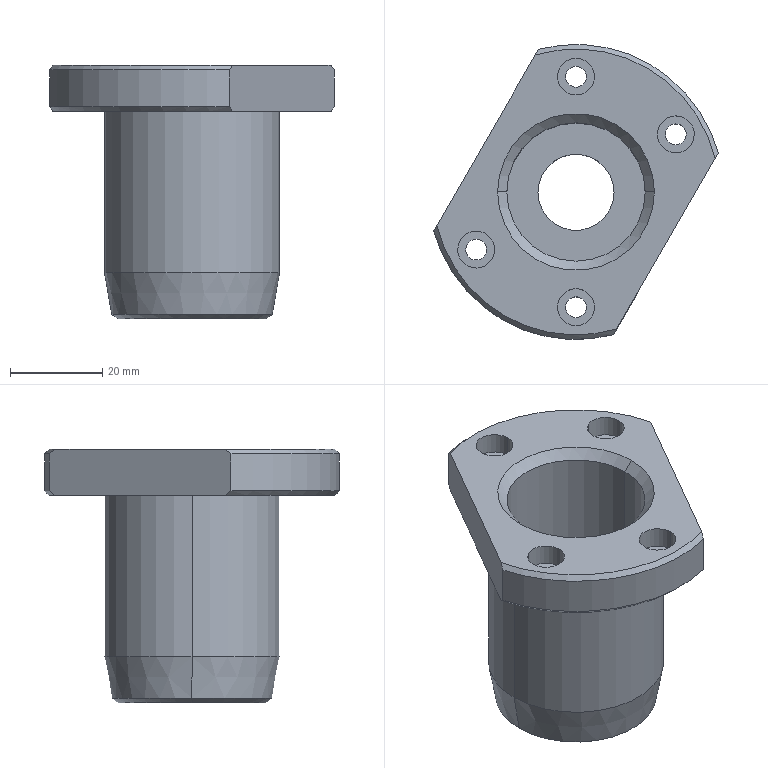Part | SolidWorks | features Chamfer 4, ICE 3, 3DProfileFeature 2, HoleWzd 2, CirPattern 1, Extrusion 1 | 1 solid | 44 faces | box 61.725 x 64 x 55 mm | volume 43113 mm3 | cylinder 24 | cone 10 | plane 10 | commonest cylinder face diameters 4.5 x8 8 x8 16.5 x2 30 x2 38 x2 64 x2
STEP:
#1=CARTESIAN_POINT('',(-15.,0.,53.));
#2=VERTEX_POINT('',#1);
#3=CARTESIAN_POINT('',(15.,0.,53.));
#4=VERTEX_POINT('',#3);
#5=CARTESIAN_POINT('',(0.,0.,53.));
#6=DIRECTION('',(0.,0.,1.));
#7=DIRECTION('',(1.,0.,0.));
#8=AXIS2_PLACEMENT_3D('',#5,#6,#7);
#9=CIRCLE('',#8,15.);
#10=EDGE_CURVE('',#2,#4,#9,.T.);
#11=ORIENTED_EDGE('',*,*,#10,.F.);
#12=CARTESIAN_POINT('',(-17.,0.,55.));
#13=VERTEX_POINT('',#12);
#14=CARTESIAN_POINT('',(-15.,0.,53.));
#15=DIRECTION('',(-0.7071,0.,0.7071));
#16=VECTOR('',#15,1000.);
#17=LINE('',#14,#16);
#18=EDGE_CURVE('',#2,#13,#17,.T.);
#19=ORIENTED_EDGE('',*,*,#18,.T.);
#20=CARTESIAN_POINT('',(17.,0.,55.));
#21=VERTEX_POINT('',#20);
#22=CARTESIAN_POINT('',(0.,0.,55.));
#23=DIRECTION('',(0.,0.,-1.));
#24=DIRECTION('',(1.,0.,0.));
#25=AXIS2_PLACEMENT_3D('',#22,#23,#24);
#26=CIRCLE('',#25,17.);
#27=EDGE_CURVE('',#21,#13,#26,.T.);
#28=ORIENTED_EDGE('',*,*,#27,.F.);
#29=CARTESIAN_POINT('',(15.,0.,53.));
#30=DIRECTION('',(0.7071,0.,0.7071));
#31=VECTOR('',#30,1000.);
#32=LINE('',#29,#31);
#33=EDGE_CURVE('',#4,#21,#32,.T.);
#34=ORIENTED_EDGE('',*,*,#33,.F.);
#35=EDGE_LOOP('',(#11,#19,#28,#34));
#36=FACE_OUTER_BOUND('',#35,.T.);
#37=CARTESIAN_POINT('',(0.,0.,53.));
#38=DIRECTION('',(0.,0.,1.));
#39=DIRECTION('',(1.,0.,0.));
#40=AXIS2_PLACEMENT_3D('',#37,#38,#39);
#41=CONICAL_SURFACE('',#40,15.,0.7854);
#42=ADVANCED_FACE('',(#36),#41,.F.);
#43=CARTESIAN_POINT('',(-16.004,0.,0.));
#44=VERTEX_POINT('',#43);
#45=CARTESIAN_POINT('',(16.004,0.,0.));
#46=VERTEX_POINT('',#45);
#47=CARTESIAN_POINT('',(0.,0.,0.));
#48=DIRECTION('',(0.,0.,-1.));
#49=DIRECTION('',(1.,0.,0.));
#50=AXIS2_PLACEMENT_3D('',#47,#48,#49);
#51=CIRCLE('',#50,16.004);
#52=EDGE_CURVE('',#44,#46,#51,.T.);
#53=ORIENTED_EDGE('',*,*,#52,.F.);
#54=CARTESIAN_POINT('',(-17.41,0.,0.9848));
#55=VERTEX_POINT('',#54);
#56=CARTESIAN_POINT('',(-16.004,0.,0.));
#57=DIRECTION('',(-0.8192,0.,0.5736));
#58=VECTOR('',#57,1000.);
#59=LINE('',#56,#58);
#60=EDGE_CURVE('',#44,#55,#59,.T.);
#61=ORIENTED_EDGE('',*,*,#60,.T.);
#62=CARTESIAN_POINT('',(17.41,0.,0.9848));
#63=VERTEX_POINT('',#62);
#64=CARTESIAN_POINT('',(0.,0.,0.9848));
#65=DIRECTION('',(0.,0.,1.));
#66=DIRECTION('',(1.,0.,0.));
#67=AXIS2_PLACEMENT_3D('',#64,#65,#66);
#68=CIRCLE('',#67,17.41);
#69=EDGE_CURVE('',#63,#55,#68,.T.);
#70=ORIENTED_EDGE('',*,*,#69,.F.);
#71=CARTESIAN_POINT('',(16.004,0.,0.));
#72=DIRECTION('',(0.8192,0.,0.5736));
#73=VECTOR('',#72,1000.);
#74=LINE('',#71,#73);
#75=EDGE_CURVE('',#46,#63,#74,.T.);
#76=ORIENTED_EDGE('',*,*,#75,.F.);
#77=EDGE_LOOP('',(#53,#61,#70,#76));
#78=FACE_OUTER_BOUND('',#77,.T.);
#79=CARTESIAN_POINT('',(0.,0.,0.));
#80=DIRECTION('',(0.,0.,1.));
#81=DIRECTION('',(1.,0.,0.));
#82=AXIS2_PLACEMENT_3D('',#79,#80,#81);
#83=CONICAL_SURFACE('',#82,16.004,0.9599);
#84=ADVANCED_FACE('',(#78),#83,.T.);
#85=ORIENTED_EDGE('',*,*,#69,.T.);
#86=CARTESIAN_POINT('',(-19.,0.,10.));
#87=VERTEX_POINT('',#86);
#88=CARTESIAN_POINT('',(-19.,0.,10.));
#89=DIRECTION('',(-0.1736,0.,0.9848));
#90=VECTOR('',#89,1000.);
#91=LINE('',#88,#90);
#92=EDGE_CURVE('',#55,#87,#91,.T.);
#93=ORIENTED_EDGE('',*,*,#92,.T.);
#94=CARTESIAN_POINT('',(19.,0.,10.));
#95=VERTEX_POINT('',#94);
#96=CARTESIAN_POINT('',(0.,0.,10.));
#97=DIRECTION('',(0.,0.,1.));
#98=DIRECTION('',(1.,0.,0.));
#99=AXIS2_PLACEMENT_3D('',#96,#97,#98);
#100=CIRCLE('',#99,19.);
#101=EDGE_CURVE('',#95,#87,#100,.T.);
#102=ORIENTED_EDGE('',*,*,#101,.F.);
#103=CARTESIAN_POINT('',(19.,0.,10.));
#104=DIRECTION('',(0.1736,0.,0.9848));
#105=VECTOR('',#104,1000.);
#106=LINE('',#103,#105);
#107=EDGE_CURVE('',#63,#95,#106,.T.);
#108=ORIENTED_EDGE('',*,*,#107,.F.);
#109=EDGE_LOOP('',(#85,#93,#102,#108));
#110=FACE_OUTER_BOUND('',#109,.T.);
#111=CARTESIAN_POINT('',(0.,0.,10.));
#112=DIRECTION('',(0.,0.,1.));
#113=DIRECTION('',(1.,0.,0.));
#114=AXIS2_PLACEMENT_3D('',#111,#112,#113);
#115=CONICAL_SURFACE('',#114,19.,0.1745);
#116=ADVANCED_FACE('',(#110),#115,.T.);
#117=CARTESIAN_POINT('',(19.651,15.964,50.4));
#118=VERTEX_POINT('',#117);
#119=CARTESIAN_POINT('',(23.651,9.036,50.4));
#120=VERTEX_POINT('',#119);
#121=CARTESIAN_POINT('',(21.651,12.5,50.4));
#122=DIRECTION('',(0.,0.,1.));
#123=DIRECTION('',(0.5,-0.866,0.));
#124=AXIS2_PLACEMENT_3D('',#121,#122,#123);
#125=CIRCLE('',#124,4.);
#126=EDGE_CURVE('',#118,#120,#125,.T.);
#127=ORIENTED_EDGE('',*,*,#126,.F.);
#128=CARTESIAN_POINT('',(19.651,15.964,55.));
#129=VERTEX_POINT('',#128);
#130=CARTESIAN_POINT('',(19.651,15.964,55.));
#131=DIRECTION('',(0.,0.,1.));
#132=VECTOR('',#131,1000.);
#133=LINE('',#130,#132);
#134=EDGE_CURVE('',#118,#129,#133,.T.);
#135=ORIENTED_EDGE('',*,*,#134,.T.);
#136=CARTESIAN_POINT('',(23.651,9.036,55.));
#137=VERTEX_POINT('',#136);
#138=CARTESIAN_POINT('',(21.651,12.5,55.));
#139=DIRECTION('',(0.,0.,1.));
#140=DIRECTION('',(0.5,-0.866,0.));
#141=AXIS2_PLACEMENT_3D('',#138,#139,#140);
#142=CIRCLE('',#141,4.);
#143=EDGE_CURVE('',#129,#137,#142,.T.);
#144=ORIENTED_EDGE('',*,*,#143,.T.);
#145=CARTESIAN_POINT('',(23.651,9.036,55.));
#146=DIRECTION('',(0.,0.,1.));
#147=VECTOR('',#146,1000.);
#148=LINE('',#145,#147);
#149=EDGE_CURVE('',#120,#137,#148,.T.);
#150=ORIENTED_EDGE('',*,*,#149,.F.);
#151=EDGE_LOOP('',(#127,#135,#144,#150));
#152=FACE_OUTER_BOUND('',#151,.T.);
#153=CARTESIAN_POINT('',(21.651,12.5,55.));
#154=DIRECTION('',(0.,0.,1.));
#155=DIRECTION('',(0.5,-0.866,0.));
#156=AXIS2_PLACEMENT_3D('',#153,#154,#155);
#157=CYLINDRICAL_SURFACE('',#156,4.);
#158=ADVANCED_FACE('',(#152),#157,.F.);
#159=CARTESIAN_POINT('',(20.526,14.449,45.));
#160=VERTEX_POINT('',#159);
#161=CARTESIAN_POINT('',(22.776,10.551,45.));
#162=VERTEX_POINT('',#161);
#163=CARTESIAN_POINT('',(21.651,12.5,45.));
#164=DIRECTION('',(0.,0.,1.));
#165=DIRECTION('',(0.5,-0.866,0.));
#166=AXIS2_PLACEMENT_3D('',#163,#164,#165);
#167=CIRCLE('',#166,2.25);
#168=EDGE_CURVE('',#160,#162,#167,.T.);
#169=ORIENTED_EDGE('',*,*,#168,.F.);
#170=CARTESIAN_POINT('',(20.526,14.449,50.4));
#171=VERTEX_POINT('',#170);
#172=CARTESIAN_POINT('',(20.526,14.449,55.));
#173=DIRECTION('',(0.,0.,1.));
#174=VECTOR('',#173,1000.);
#175=LINE('',#172,#174);
#176=EDGE_CURVE('',#160,#171,#175,.T.);
#177=ORIENTED_EDGE('',*,*,#176,.T.);
#178=CARTESIAN_POINT('',(22.776,10.551,50.4));
#179=VERTEX_POINT('',#178);
#180=CARTESIAN_POINT('',(21.651,12.5,50.4));
#181=DIRECTION('',(0.,0.,1.));
#182=DIRECTION('',(0.5,-0.866,0.));
#183=AXIS2_PLACEMENT_3D('',#180,#181,#182);
#184=CIRCLE('',#183,2.25);
#185=EDGE_CURVE('',#171,#179,#184,.T.);
#186=ORIENTED_EDGE('',*,*,#185,.T.);
#187=CARTESIAN_POINT('',(22.776,10.551,55.));
#188=DIRECTION('',(0.,0.,1.));
#189=VECTOR('',#188,1000.);
#190=LINE('',#187,#189);
#191=EDGE_CURVE('',#162,#179,#190,.T.);
#192=ORIENTED_EDGE('',*,*,#191,.F.);
#193=EDGE_LOOP('',(#169,#177,#186,#192));
#194=FACE_OUTER_BOUND('',#193,.T.);
#195=CARTESIAN_POINT('',(21.651,12.5,55.));
#196=DIRECTION('',(0.,0.,1.));
#197=DIRECTION('',(0.5,-0.866,0.));
#198=AXIS2_PLACEMENT_3D('',#195,#196,#197);
#199=CYLINDRICAL_SURFACE('',#198,2.25);
#200=ADVANCED_FACE('',(#194),#199,.F.);
#201=CARTESIAN_POINT('',(4.,-25.,50.4));
#202=VERTEX_POINT('',#201);
#203=CARTESIAN_POINT('',(-4.,-25.,50.4));
#204=VERTEX_POINT('',#203);
#205=CARTESIAN_POINT('',(0.,-25.,50.4));
#206=DIRECTION('',(0.,0.,1.));
#207=DIRECTION('',(-1.,0.,0.));
#208=AXIS2_PLACEMENT_3D('',#205,#206,#207);
#209=CIRCLE('',#208,4.);
#210=EDGE_CURVE('',#202,#204,#209,.T.);
#211=ORIENTED_EDGE('',*,*,#210,.F.);
#212=CARTESIAN_POINT('',(4.,-25.,55.));
#213=VERTEX_POINT('',#212);
#214=CARTESIAN_POINT('',(4.,-25.,55.));
#215=DIRECTION('',(0.,0.,1.));
#216=VECTOR('',#215,1000.);
#217=LINE('',#214,#216);
#218=EDGE_CURVE('',#202,#213,#217,.T.);
#219=ORIENTED_EDGE('',*,*,#218,.T.);
#220=CARTESIAN_POINT('',(-4.,-25.,55.));
#221=VERTEX_POINT('',#220);
#222=CARTESIAN_POINT('',(0.,-25.,55.));
#223=DIRECTION('',(0.,0.,1.));
#224=DIRECTION('',(-1.,0.,0.));
#225=AXIS2_PLACEMENT_3D('',#222,#223,#224);
#226=CIRCLE('',#225,4.);
#227=EDGE_CURVE('',#213,#221,#226,.T.);
#228=ORIENTED_EDGE('',*,*,#227,.T.);
#229=CARTESIAN_POINT('',(-4.,-25.,55.));
#230=DIRECTION('',(0.,0.,1.));
#231=VECTOR('',#230,1000.);
#232=LINE('',#229,#231);
#233=EDGE_CURVE('',#204,#221,#232,.T.);
#234=ORIENTED_EDGE('',*,*,#233,.F.);
#235=EDGE_LOOP('',(#211,#219,#228,#234));
#236=FACE_OUTER_BOUND('',#235,.T.);
#237=CARTESIAN_POINT('',(0.,-25.,55.));
#238=DIRECTION('',(0.,0.,1.));
#239=DIRECTION('',(-1.,0.,0.));
#240=AXIS2_PLACEMENT_3D('',#237,#238,#239);
#241=CYLINDRICAL_SURFACE('',#240,4.);
#242=ADVANCED_FACE('',(#236),#241,.F.);
#243=CARTESIAN_POINT('',(2.25,-25.,45.));
#244=VERTEX_POINT('',#243);
#245=CARTESIAN_POINT('',(-2.25,-25.,45.));
#246=VERTEX_POINT('',#245);
#247=CARTESIAN_POINT('',(0.,-25.,45.));
#248=DIRECTION('',(0.,0.,1.));
#249=DIRECTION('',(-1.,0.,0.));
#250=AXIS2_PLACEMENT_3D('',#247,#248,#249);
#251=CIRCLE('',#250,2.25);
#252=EDGE_CURVE('',#244,#246,#251,.T.);
#253=ORIENTED_EDGE('',*,*,#252,.F.);
#254=CARTESIAN_POINT('',(2.25,-25.,50.4));
#255=VERTEX_POINT('',#254);
#256=CARTESIAN_POINT('',(2.25,-25.,55.));
#257=DIRECTION('',(0.,0.,1.));
#258=VECTOR('',#257,1000.);
#259=LINE('',#256,#258);
#260=EDGE_CURVE('',#244,#255,#259,.T.);
#261=ORIENTED_EDGE('',*,*,#260,.T.);
#262=CARTESIAN_POINT('',(-2.25,-25.,50.4));
#263=VERTEX_POINT('',#262);
#264=CARTESIAN_POINT('',(0.,-25.,50.4));
#265=DIRECTION('',(0.,0.,1.));
#266=DIRECTION('',(-1.,0.,0.));
#267=AXIS2_PLACEMENT_3D('',#264,#265,#266);
#268=CIRCLE('',#267,2.25);
#269=EDGE_CURVE('',#255,#263,#268,.T.);
#270=ORIENTED_EDGE('',*,*,#269,.T.);
#271=CARTESIAN_POINT('',(-2.25,-25.,55.));
#272=DIRECTION('',(0.,0.,1.));
#273=VECTOR('',#272,1000.);
#274=LINE('',#271,#273);
#275=EDGE_CURVE('',#246,#263,#274,.T.);
#276=ORIENTED_EDGE('',*,*,#275,.F.);
#277=EDGE_LOOP('',(#253,#261,#270,#276));
#278=FACE_OUTER_BOUND('',#277,.T.);
#279=CARTESIAN_POINT('',(0.,-25.,55.));
#280=DIRECTION('',(0.,0.,1.));
#281=DIRECTION('',(-1.,0.,0.));
#282=AXIS2_PLACEMENT_3D('',#279,#280,#281);
#283=CYLINDRICAL_SURFACE('',#282,2.25);
#284=ADVANCED_FACE('',(#278),#283,.F.);
#285=CARTESIAN_POINT('',(-19.651,-15.964,50.4));
#286=VERTEX_POINT('',#285);
#287=CARTESIAN_POINT('',(-23.651,-9.036,50.4));
#288=VERTEX_POINT('',#287);
#289=CARTESIAN_POINT('',(-21.651,-12.5,50.4));
#290=DIRECTION('',(0.,0.,1.));
#291=DIRECTION('',(-0.5,0.866,0.));
#292=AXIS2_PLACEMENT_3D('',#289,#290,#291);
#293=CIRCLE('',#292,4.);
#294=EDGE_CURVE('',#286,#288,#293,.T.);
#295=ORIENTED_EDGE('',*,*,#294,.F.);
#296=CARTESIAN_POINT('',(-19.651,-15.964,55.));
#297=VERTEX_POINT('',#296);
#298=CARTESIAN_POINT('',(-19.651,-15.964,55.));
#299=DIRECTION('',(0.,0.,1.));
#300=VECTOR('',#299,1000.);
#301=LINE('',#298,#300);
#302=EDGE_CURVE('',#286,#297,#301,.T.);
#303=ORIENTED_EDGE('',*,*,#302,.T.);
#304=CARTESIAN_POINT('',(-23.651,-9.036,55.));
#305=VERTEX_POINT('',#304);
#306=CARTESIAN_POINT('',(-21.651,-12.5,55.));
#307=DIRECTION('',(0.,0.,1.));
#308=DIRECTION('',(-0.5,0.866,0.));
#309=AXIS2_PLACEMENT_3D('',#306,#307,#308);
#310=CIRCLE('',#309,4.);
#311=EDGE_CURVE('',#297,#305,#310,.T.);
#312=ORIENTED_EDGE('',*,*,#311,.T.);
#313=CARTESIAN_POINT('',(-23.651,-9.036,55.));
#314=DIRECTION('',(0.,0.,1.));
#315=VECTOR('',#314,1000.);
#316=LINE('',#313,#315);
#317=EDGE_CURVE('',#288,#305,#316,.T.);
#318=ORIENTED_EDGE('',*,*,#317,.F.);
#319=EDGE_LOOP('',(#295,#303,#312,#318));
#320=FACE_OUTER_BOUND('',#319,.T.);
#321=CARTESIAN_POINT('',(-21.651,-12.5,55.));
#322=DIRECTION('',(0.,0.,1.));
#323=DIRECTION('',(-0.5,0.866,0.));
#324=AXIS2_PLACEMENT_3D('',#321,#322,#323);
#325=CYLINDRICAL_SURFACE('',#324,4.);
#326=ADVANCED_FACE('',(#320),#325,.F.);
#327=CARTESIAN_POINT('',(-20.526,-14.449,45.));
#328=VERTEX_POINT('',#327);
#329=CARTESIAN_POINT('',(-22.776,-10.551,45.));
#330=VERTEX_POINT('',#329);
#331=CARTESIAN_POINT('',(-21.651,-12.5,45.));
#332=DIRECTION('',(0.,0.,1.));
#333=DIRECTION('',(-0.5,0.866,0.));
#334=AXIS2_PLACEMENT_3D('',#331,#332,#333);
#335=CIRCLE('',#334,2.25);
#336=EDGE_CURVE('',#328,#330,#335,.T.);
#337=ORIENTED_EDGE('',*,*,#336,.F.);
#338=CARTESIAN_POINT('',(-20.526,-14.449,50.4));
#339=VERTEX_POINT('',#338);
#340=CARTESIAN_POINT('',(-20.526,-14.449,55.));
#341=DIRECTION('',(0.,0.,1.));
#342=VECTOR('',#341,1000.);
#343=LINE('',#340,#342);
#344=EDGE_CURVE('',#328,#339,#343,.T.);
#345=ORIENTED_EDGE('',*,*,#344,.T.);
#346=CARTESIAN_POINT('',(-22.776,-10.551,50.4));
#347=VERTEX_POINT('',#346);
#348=CARTESIAN_POINT('',(-21.651,-12.5,50.4));
#349=DIRECTION('',(0.,0.,1.));
#350=DIRECTION('',(-0.5,0.866,0.));
#351=AXIS2_PLACEMENT_3D('',#348,#349,#350);
#352=CIRCLE('',#351,2.25);
#353=EDGE_CURVE('',#339,#347,#352,.T.);
#354=ORIENTED_EDGE('',*,*,#353,.T.);
#355=CARTESIAN_POINT('',(-22.776,-10.551,55.));
#356=DIRECTION('',(0.,0.,1.));
#357=VECTOR('',#356,1000.);
#358=LINE('',#355,#357);
#359=EDGE_CURVE('',#330,#347,#358,.T.);
#360=ORIENTED_EDGE('',*,*,#359,.F.);
#361=EDGE_LOOP('',(#337,#345,#354,#360));
#362=FACE_OUTER_BOUND('',#361,.T.);
#363=CARTESIAN_POINT('',(-21.651,-12.5,55.));
#364=DIRECTION('',(0.,0.,1.));
#365=DIRECTION('',(-0.5,0.866,0.));
#366=AXIS2_PLACEMENT_3D('',#363,#364,#365);
#367=CYLINDRICAL_SURFACE('',#366,2.25);
#368=ADVANCED_FACE('',(#362),#367,.F.);
#369=CARTESIAN_POINT('',(-4.,25.,50.4));
#370=VERTEX_POINT('',#369);
#371=CARTESIAN_POINT('',(4.,25.,50.4));
#372=VERTEX_POINT('',#371);
#373=CARTESIAN_POINT('',(0.,25.,50.4));
#374=DIRECTION('',(0.,0.,1.));
#375=DIRECTION('',(1.,0.,0.));
#376=AXIS2_PLACEMENT_3D('',#373,#374,#375);
#377=CIRCLE('',#376,4.);
#378=EDGE_CURVE('',#370,#372,#377,.T.);
#379=ORIENTED_EDGE('',*,*,#378,.F.);
#380=CARTESIAN_POINT('',(-4.,25.,55.));
#381=VERTEX_POINT('',#380);
#382=CARTESIAN_POINT('',(-4.,25.,55.));
#383=DIRECTION('',(0.,0.,1.));
#384=VECTOR('',#383,1000.);
#385=LINE('',#382,#384);
#386=EDGE_CURVE('',#370,#381,#385,.T.);
#387=ORIENTED_EDGE('',*,*,#386,.T.);
#388=CARTESIAN_POINT('',(4.,25.,55.));
#389=VERTEX_POINT('',#388);
#390=CARTESIAN_POINT('',(0.,25.,55.));
#391=DIRECTION('',(0.,0.,1.));
#392=DIRECTION('',(1.,0.,0.));
#393=AXIS2_PLACEMENT_3D('',#390,#391,#392);
#394=CIRCLE('',#393,4.);
#395=EDGE_CURVE('',#381,#389,#394,.T.);
#396=ORIENTED_EDGE('',*,*,#395,.T.);
#397=CARTESIAN_POINT('',(4.,25.,55.));
#398=DIRECTION('',(0.,0.,1.));
#399=VECTOR('',#398,1000.);
#400=LINE('',#397,#399);
#401=EDGE_CURVE('',#372,#389,#400,.T.);
#402=ORIENTED_EDGE('',*,*,#401,.F.);
#403=EDGE_LOOP('',(#379,#387,#396,#402));
#404=FACE_OUTER_BOUND('',#403,.T.);
#405=CARTESIAN_POINT('',(0.,25.,55.));
#406=DIRECTION('',(0.,0.,1.));
#407=DIRECTION('',(1.,0.,0.));
#408=AXIS2_PLACEMENT_3D('',#405,#406,#407);
#409=CYLINDRICAL_SURFACE('',#408,4.);
#410=ADVANCED_FACE('',(#404),#409,.F.);
#411=CARTESIAN_POINT('',(-2.25,25.,45.));
#412=VERTEX_POINT('',#411);
#413=CARTESIAN_POINT('',(2.25,25.,45.));
#414=VERTEX_POINT('',#413);
#415=CARTESIAN_POINT('',(0.,25.,45.));
#416=DIRECTION('',(0.,0.,1.));
#417=DIRECTION('',(1.,0.,0.));
#418=AXIS2_PLACEMENT_3D('',#415,#416,#417);
#419=CIRCLE('',#418,2.25);
#420=EDGE_CURVE('',#412,#414,#419,.T.);
#421=ORIENTED_EDGE('',*,*,#420,.F.);
#422=CARTESIAN_POINT('',(-2.25,25.,50.4));
#423=VERTEX_POINT('',#422);
#424=CARTESIAN_POINT('',(-2.25,25.,55.));
#425=DIRECTION('',(0.,0.,1.));
#426=VECTOR('',#425,1000.);
#427=LINE('',#424,#426);
#428=EDGE_CURVE('',#412,#423,#427,.T.);
#429=ORIENTED_EDGE('',*,*,#428,.T.);
#430=CARTESIAN_POINT('',(2.25,25.,50.4));
#431=VERTEX_POINT('',#430);
#432=CARTESIAN_POINT('',(0.,25.,50.4));
#433=DIRECTION('',(0.,0.,1.));
#434=DIRECTION('',(1.,0.,0.));
#435=AXIS2_PLACEMENT_3D('',#432,#433,#434);
#436=CIRCLE('',#435,2.25);
#437=EDGE_CURVE('',#423,#431,#436,.T.);
#438=ORIENTED_EDGE('',*,*,#437,.T.);
#439=CARTESIAN_POINT('',(2.25,25.,55.));
#440=DIRECTION('',(0.,0.,1.));
#441=VECTOR('',#440,1000.);
#442=LINE('',#439,#441);
#443=EDGE_CURVE('',#414,#431,#442,.T.);
#444=ORIENTED_EDGE('',*,*,#443,.F.);
#445=EDGE_LOOP('',(#421,#429,#438,#444));
#446=FACE_OUTER_BOUND('',#445,.T.);
#447=CARTESIAN_POINT('',(0.,25.,55.));
#448=DIRECTION('',(0.,0.,1.));
#449=DIRECTION('',(1.,0.,0.));
#450=AXIS2_PLACEMENT_3D('',#447,#448,#449);
#451=CYLINDRICAL_SURFACE('',#450,2.25);
#452=ADVANCED_FACE('',(#446),#451,.F.);
#453=CARTESIAN_POINT('',(-8.25,0.,15.));
#454=VERTEX_POINT('',#453);
#455=CARTESIAN_POINT('',(8.25,0.,15.));
#456=VERTEX_POINT('',#455);
#457=CARTESIAN_POINT('',(0.,0.,15.));
#458=DIRECTION('',(0.,0.,1.));
#459=DIRECTION('',(1.,0.,0.));
#460=AXIS2_PLACEMENT_3D('',#457,#458,#459);
#461=CIRCLE('',#460,8.25);
#462=EDGE_CURVE('',#454,#456,#461,.T.);
#463=ORIENTED_EDGE('',*,*,#462,.T.);
#464=CARTESIAN_POINT('',(8.25,0.,0.));
#465=VERTEX_POINT('',#464);
#466=CARTESIAN_POINT('',(8.25,0.,0.));
#467=DIRECTION('',(0.,0.,-1.));
#468=VECTOR('',#467,1000.);
#469=LINE('',#466,#468);
#470=EDGE_CURVE('',#456,#465,#469,.T.);
#471=ORIENTED_EDGE('',*,*,#470,.T.);
#472=CARTESIAN_POINT('',(-8.25,0.,0.));
#473=VERTEX_POINT('',#472);
#474=CARTESIAN_POINT('',(0.,0.,0.));
#475=DIRECTION('',(0.,0.,-1.));
#476=DIRECTION('',(-1.,0.,0.));
#477=AXIS2_PLACEMENT_3D('',#474,#475,#476);
#478=CIRCLE('',#477,8.25);
#479=EDGE_CURVE('',#465,#473,#478,.T.);
#480=ORIENTED_EDGE('',*,*,#479,.T.);
#481=CARTESIAN_POINT('',(-8.25,0.,0.));
#482=DIRECTION('',(0.,0.,-1.));
#483=VECTOR('',#482,1000.);
#484=LINE('',#481,#483);
#485=EDGE_CURVE('',#454,#473,#484,.T.);
#486=ORIENTED_EDGE('',*,*,#485,.F.);
#487=EDGE_LOOP('',(#463,#471,#480,#486));
#488=FACE_OUTER_BOUND('',#487,.T.);
#489=CARTESIAN_POINT('',(0.,0.,0.));
#490=DIRECTION('',(0.,0.,-1.));
#491=DIRECTION('',(-1.,0.,0.));
#492=AXIS2_PLACEMENT_3D('',#489,#490,#491);
#493=CYLINDRICAL_SURFACE('',#492,8.25);
#494=ADVANCED_FACE('',(#488),#493,.F.);
#495=CARTESIAN_POINT('',(15.,0.,15.));
#496=VERTEX_POINT('',#495);
#497=CARTESIAN_POINT('',(-15.,0.,15.));
#498=VERTEX_POINT('',#497);
#499=CARTESIAN_POINT('',(0.,0.,15.));
#500=DIRECTION('',(0.,0.,-1.));
#501=DIRECTION('',(1.,0.,0.));
#502=AXIS2_PLACEMENT_3D('',#499,#500,#501);
#503=CIRCLE('',#502,15.);
#504=EDGE_CURVE('',#496,#498,#503,.T.);
#505=ORIENTED_EDGE('',*,*,#504,.T.);
#506=CARTESIAN_POINT('',(-15.,0.,-42.426));
#507=DIRECTION('',(0.,0.,1.));
#508=VECTOR('',#507,1000.);
#509=LINE('',#506,#508);
#510=EDGE_CURVE('',#498,#2,#509,.T.);
#511=ORIENTED_EDGE('',*,*,#510,.T.);
#512=ORIENTED_EDGE('',*,*,#10,.T.);
#513=CARTESIAN_POINT('',(15.,0.,-42.426));
#514=DIRECTION('',(0.,0.,1.));
#515=VECTOR('',#514,1000.);
#516=LINE('',#513,#515);
#517=EDGE_CURVE('',#496,#4,#516,.T.);
#518=ORIENTED_EDGE('',*,*,#517,.F.);
#519=EDGE_LOOP('',(#505,#511,#512,#518));
#520=FACE_OUTER_BOUND('',#519,.T.);
#521=CARTESIAN_POINT('',(0.,0.,-42.426));
#522=DIRECTION('',(0.,0.,1.));
#523=DIRECTION('',(1.,0.,0.));
#524=AXIS2_PLACEMENT_3D('',#521,#522,#523);
#525=CYLINDRICAL_SURFACE('',#524,15.);
#526=ADVANCED_FACE('',(#520),#525,.F.);
#527=CARTESIAN_POINT('',(19.,0.,45.));
#528=VERTEX_POINT('',#527);
#529=CARTESIAN_POINT('',(-19.,0.,45.));
#530=VERTEX_POINT('',#529);
#531=CARTESIAN_POINT('',(0.,0.,45.));
#532=DIRECTION('',(0.,0.,1.));
#533=DIRECTION('',(1.,0.,0.));
#534=AXIS2_PLACEMENT_3D('',#531,#532,#533);
#535=CIRCLE('',#534,19.);
#536=EDGE_CURVE('',#528,#530,#535,.T.);
#537=ORIENTED_EDGE('',*,*,#536,.F.);
#538=CARTESIAN_POINT('',(19.,0.,45.));
#539=DIRECTION('',(0.,0.,-1.));
#540=VECTOR('',#539,1000.);
#541=LINE('',#538,#540);
#542=EDGE_CURVE('',#528,#95,#541,.T.);
#543=ORIENTED_EDGE('',*,*,#542,.T.);
#544=ORIENTED_EDGE('',*,*,#101,.T.);
#545=CARTESIAN_POINT('',(-19.,0.,45.));
#546=DIRECTION('',(0.,0.,-1.));
#547=VECTOR('',#546,1000.);
#548=LINE('',#545,#547);
#549=EDGE_CURVE('',#530,#87,#548,.T.);
#550=ORIENTED_EDGE('',*,*,#549,.F.);
#551=EDGE_LOOP('',(#537,#543,#544,#550));
#552=FACE_OUTER_BOUND('',#551,.T.);
#553=CARTESIAN_POINT('',(0.,0.,45.));
#554=DIRECTION('',(0.,0.,-1.));
#555=DIRECTION('',(-1.,0.,0.));
#556=AXIS2_PLACEMENT_3D('',#553,#554,#555);
#557=CYLINDRICAL_SURFACE('',#556,19.);
#558=ADVANCED_FACE('',(#552),#557,.T.);
#559=CARTESIAN_POINT('',(30.863,8.456,46.));
#560=VERTEX_POINT('',#559);
#561=CARTESIAN_POINT('',(30.863,8.456,54.));
#562=VERTEX_POINT('',#561);
#563=CARTESIAN_POINT('',(30.863,8.456,-0.001));
#564=DIRECTION('',(0.,0.,1.));
#565=VECTOR('',#564,1000.);
#566=LINE('',#563,#565);
#567=EDGE_CURVE('',#560,#562,#566,.T.);
#568=ORIENTED_EDGE('',*,*,#567,.F.);
#569=CARTESIAN_POINT('',(-8.109,30.956,46.));
#570=VERTEX_POINT('',#569);
#571=CARTESIAN_POINT('',(0.,0.,46.));
#572=DIRECTION('',(0.,0.,1.));
#573=DIRECTION('',(1.,0.,0.));
#574=AXIS2_PLACEMENT_3D('',#571,#572,#573);
#575=CIRCLE('',#574,32.);
#576=EDGE_CURVE('',#560,#570,#575,.T.);
#577=ORIENTED_EDGE('',*,*,#576,.T.);
#578=CARTESIAN_POINT('',(-8.109,30.956,54.));
#579=VERTEX_POINT('',#578);
#580=CARTESIAN_POINT('',(-8.109,30.956,-0.001));
#581=DIRECTION('',(0.,0.,1.));
#582=VECTOR('',#581,1000.);
#583=LINE('',#580,#582);
#584=EDGE_CURVE('',#570,#579,#583,.T.);
#585=ORIENTED_EDGE('',*,*,#584,.T.);
#586=CARTESIAN_POINT('',(0.,0.,54.));
#587=DIRECTION('',(0.,0.,-1.));
#588=DIRECTION('',(1.,0.,0.));
#589=AXIS2_PLACEMENT_3D('',#586,#587,#588);
#590=CIRCLE('',#589,32.);
#591=EDGE_CURVE('',#579,#562,#590,.T.);
#592=ORIENTED_EDGE('',*,*,#591,.T.);
#593=EDGE_LOOP('',(#568,#577,#585,#592));
#594=FACE_OUTER_BOUND('',#593,.T.);
#595=CARTESIAN_POINT('',(0.,0.,55.));
#596=DIRECTION('',(0.,0.,-1.));
#597=DIRECTION('',(-1.,0.,0.));
#598=AXIS2_PLACEMENT_3D('',#595,#596,#597);
#599=CYLINDRICAL_SURFACE('',#598,32.);
#600=ADVANCED_FACE('',(#594),#599,.T.);
#601=ORIENTED_EDGE('',*,*,#542,.F.);
#602=CARTESIAN_POINT('',(0.,0.,45.));
#603=DIRECTION('',(0.,0.,1.));
#604=DIRECTION('',(1.,0.,0.));
#605=AXIS2_PLACEMENT_3D('',#602,#603,#604);
#606=CIRCLE('',#605,19.);
#607=EDGE_CURVE('',#530,#528,#606,.T.);
#608=ORIENTED_EDGE('',*,*,#607,.F.);
#609=ORIENTED_EDGE('',*,*,#549,.T.);
#610=CARTESIAN_POINT('',(0.,0.,10.));
#611=DIRECTION('',(0.,0.,1.));
#612=DIRECTION('',(1.,0.,0.));
#613=AXIS2_PLACEMENT_3D('',#610,#611,#612);
#614=CIRCLE('',#613,19.);
#615=EDGE_CURVE('',#87,#95,#614,.T.);
#616=ORIENTED_EDGE('',*,*,#615,.T.);
#617=EDGE_LOOP('',(#601,#608,#609,#616));
#618=FACE_OUTER_BOUND('',#617,.T.);
#619=CARTESIAN_POINT('',(0.,0.,45.));
#620=DIRECTION('',(0.,0.,-1.));
#621=DIRECTION('',(-1.,0.,0.));
#622=AXIS2_PLACEMENT_3D('',#619,#620,#621);
#623=CYLINDRICAL_SURFACE('',#622,19.);
#624=ADVANCED_FACE('',(#618),#623,.T.);
#625=CARTESIAN_POINT('',(0.,0.,0.));
#626=DIRECTION('',(0.,0.,-1.));
#627=DIRECTION('',(1.,0.,0.));
#628=AXIS2_PLACEMENT_3D('',#625,#626,#627);
#629=CIRCLE('',#628,16.004);
#630=EDGE_CURVE('',#46,#44,#629,.T.);
#631=ORIENTED_EDGE('',*,*,#630,.T.);
#632=ORIENTED_EDGE('',*,*,#52,.T.);
#633=EDGE_LOOP('',(#631,#632));
#634=FACE_OUTER_BOUND('',#633,.T.);
#635=CARTESIAN_POINT('',(0.,0.,0.));
#636=DIRECTION('',(0.,0.,-1.));
#637=DIRECTION('',(-1.,0.,0.));
#638=AXIS2_PLACEMENT_3D('',#635,#636,#637);
#639=CIRCLE('',#638,8.25);
#640=EDGE_CURVE('',#473,#465,#639,.T.);
#641=ORIENTED_EDGE('',*,*,#640,.F.);
#642=ORIENTED_EDGE('',*,*,#479,.F.);
#643=EDGE_LOOP('',(#641,#642));
#644=FACE_BOUND('',#643,.T.);
#645=CARTESIAN_POINT('',(0.,0.,0.));
#646=DIRECTION('',(0.,0.,1.));
#647=DIRECTION('',(1.,0.,0.));
#648=AXIS2_PLACEMENT_3D('',#645,#646,#647);
#649=PLANE('',#648);
#650=ADVANCED_FACE('',(#634,#644),#649,.F.);
#651=ORIENTED_EDGE('',*,*,#510,.F.);
#652=CARTESIAN_POINT('',(0.,0.,15.));
#653=DIRECTION('',(0.,0.,-1.));
#654=DIRECTION('',(1.,0.,0.));
#655=AXIS2_PLACEMENT_3D('',#652,#653,#654);
#656=CIRCLE('',#655,15.);
#657=EDGE_CURVE('',#498,#496,#656,.T.);
#658=ORIENTED_EDGE('',*,*,#657,.T.);
#659=ORIENTED_EDGE('',*,*,#517,.T.);
#660=CARTESIAN_POINT('',(0.,0.,53.));
#661=DIRECTION('',(0.,0.,1.));
#662=DIRECTION('',(1.,0.,0.));
#663=AXIS2_PLACEMENT_3D('',#660,#661,#662);
#664=CIRCLE('',#663,15.);
#665=EDGE_CURVE('',#4,#2,#664,.T.);
#666=ORIENTED_EDGE('',*,*,#665,.T.);
#667=EDGE_LOOP('',(#651,#658,#659,#666));
#668=FACE_OUTER_BOUND('',#667,.T.);
#669=CARTESIAN_POINT('',(0.,0.,-42.426));
#670=DIRECTION('',(0.,0.,1.));
#671=DIRECTION('',(1.,0.,0.));
#672=AXIS2_PLACEMENT_3D('',#669,#670,#671);
#673=CYLINDRICAL_SURFACE('',#672,15.);
#674=ADVANCED_FACE('',(#668),#673,.F.);
#675=ORIENTED_EDGE('',*,*,#462,.F.);
#676=CARTESIAN_POINT('',(0.,0.,15.));
#677=DIRECTION('',(0.,0.,1.));
#678=DIRECTION('',(1.,0.,0.));
#679=AXIS2_PLACEMENT_3D('',#676,#677,#678);
#680=CIRCLE('',#679,8.25);
#681=EDGE_CURVE('',#456,#454,#680,.T.);
#682=ORIENTED_EDGE('',*,*,#681,.F.);
#683=EDGE_LOOP('',(#675,#682));
#684=FACE_BOUND('',#683,.T.);
#685=ORIENTED_EDGE('',*,*,#504,.F.);
#686=ORIENTED_EDGE('',*,*,#657,.F.);
#687=EDGE_LOOP('',(#685,#686));
#688=FACE_OUTER_BOUND('',#687,.T.);
#689=CARTESIAN_POINT('',(0.,0.,15.));
#690=DIRECTION('',(0.,0.,1.));
#691=DIRECTION('',(1.,0.,0.));
#692=AXIS2_PLACEMENT_3D('',#689,#690,#691);
#693=PLANE('',#692);
#694=ADVANCED_FACE('',(#684,#688),#693,.T.);
#695=ORIENTED_EDGE('',*,*,#470,.F.);
#696=ORIENTED_EDGE('',*,*,#681,.T.);
#697=ORIENTED_EDGE('',*,*,#485,.T.);
#698=ORIENTED_EDGE('',*,*,#640,.T.);
#699=EDGE_LOOP('',(#695,#696,#697,#698));
#700=FACE_OUTER_BOUND('',#699,.T.);
#701=CARTESIAN_POINT('',(0.,0.,0.));
#702=DIRECTION('',(0.,0.,-1.));
#703=DIRECTION('',(-1.,0.,0.));
#704=AXIS2_PLACEMENT_3D('',#701,#702,#703);
#705=CYLINDRICAL_SURFACE('',#704,8.25);
#706=ADVANCED_FACE('',(#700),#705,.F.);
#707=CARTESIAN_POINT('',(21.651,12.5,45.));
#708=DIRECTION('',(0.,0.,1.));
#709=DIRECTION('',(0.5,-0.866,0.));
#710=AXIS2_PLACEMENT_3D('',#707,#708,#709);
#711=CIRCLE('',#710,2.25);
#712=EDGE_CURVE('',#162,#160,#711,.T.);
#713=ORIENTED_EDGE('',*,*,#712,.T.);
#714=ORIENTED_EDGE('',*,*,#168,.T.);
#715=EDGE_LOOP('',(#713,#714));
#716=FACE_BOUND('',#715,.T.);
#717=CARTESIAN_POINT('',(0.,-25.,45.));
#718=DIRECTION('',(0.,0.,1.));
#719=DIRECTION('',(-1.,0.,0.));
#720=AXIS2_PLACEMENT_3D('',#717,#718,#719);
#721=CIRCLE('',#720,2.25);
#722=EDGE_CURVE('',#246,#244,#721,.T.);
#723=ORIENTED_EDGE('',*,*,#722,.T.);
#724=ORIENTED_EDGE('',*,*,#252,.T.);
#725=EDGE_LOOP('',(#723,#724));
#726=FACE_BOUND('',#725,.T.);
#727=CARTESIAN_POINT('',(-21.651,-12.5,45.));
#728=DIRECTION('',(0.,0.,1.));
#729=DIRECTION('',(-0.5,0.866,0.));
#730=AXIS2_PLACEMENT_3D('',#727,#728,#729);
#731=CIRCLE('',#730,2.25);
#732=EDGE_CURVE('',#330,#328,#731,.T.);
#733=ORIENTED_EDGE('',*,*,#732,.T.);
#734=ORIENTED_EDGE('',*,*,#336,.T.);
#735=EDGE_LOOP('',(#733,#734));
#736=FACE_BOUND('',#735,.T.);
#737=CARTESIAN_POINT('',(0.,25.,45.));
#738=DIRECTION('',(0.,0.,1.));
#739=DIRECTION('',(1.,0.,0.));
#740=AXIS2_PLACEMENT_3D('',#737,#738,#739);
#741=CIRCLE('',#740,2.25);
#742=EDGE_CURVE('',#414,#412,#741,.T.);
#743=ORIENTED_EDGE('',*,*,#742,.T.);
#744=ORIENTED_EDGE('',*,*,#420,.T.);
#745=EDGE_LOOP('',(#743,#744));
#746=FACE_BOUND('',#745,.T.);
#747=CARTESIAN_POINT('',(8.823,-29.718,45.));
#748=VERTEX_POINT('',#747);
#749=CARTESIAN_POINT('',(30.148,7.218,45.));
#750=VERTEX_POINT('',#749);
#751=CARTESIAN_POINT('',(30.863,8.456,45.));
#752=DIRECTION('',(0.5,0.866,0.));
#753=VECTOR('',#752,1000.);
#754=LINE('',#751,#753);
#755=EDGE_CURVE('',#748,#750,#754,.T.);
#756=ORIENTED_EDGE('',*,*,#755,.F.);
#757=CARTESIAN_POINT('',(-30.148,-7.218,45.));
#758=VERTEX_POINT('',#757);
#759=CARTESIAN_POINT('',(0.,0.,45.));
#760=DIRECTION('',(0.,0.,-1.));
#761=DIRECTION('',(1.,0.,0.));
#762=AXIS2_PLACEMENT_3D('',#759,#760,#761);
#763=CIRCLE('',#762,31.);
#764=EDGE_CURVE('',#748,#758,#763,.T.);
#765=ORIENTED_EDGE('',*,*,#764,.T.);
#766=CARTESIAN_POINT('',(-8.823,29.718,45.));
#767=VERTEX_POINT('',#766);
#768=CARTESIAN_POINT('',(-8.109,30.956,45.));
#769=DIRECTION('',(-0.5,-0.866,0.));
#770=VECTOR('',#769,1000.);
#771=LINE('',#768,#770);
#772=EDGE_CURVE('',#767,#758,#771,.T.);
#773=ORIENTED_EDGE('',*,*,#772,.F.);
#774=CARTESIAN_POINT('',(0.,0.,45.));
#775=DIRECTION('',(0.,0.,-1.));
#776=DIRECTION('',(1.,0.,0.));
#777=AXIS2_PLACEMENT_3D('',#774,#775,#776);
#778=CIRCLE('',#777,31.);
#779=EDGE_CURVE('',#767,#750,#778,.T.);
#780=ORIENTED_EDGE('',*,*,#779,.T.);
#781=EDGE_LOOP('',(#756,#765,#773,#780));
#782=FACE_OUTER_BOUND('',#781,.T.);
#783=ORIENTED_EDGE('',*,*,#607,.T.);
#784=ORIENTED_EDGE('',*,*,#536,.T.);
#785=EDGE_LOOP('',(#783,#784));
#786=FACE_BOUND('',#785,.T.);
#787=CARTESIAN_POINT('',(0.,0.,45.));
#788=DIRECTION('',(0.,0.,1.));
#789=DIRECTION('',(1.,0.,0.));
#790=AXIS2_PLACEMENT_3D('',#787,#788,#789);
#791=PLANE('',#790);
#792=ADVANCED_FACE('',(#716,#726,#736,#746,#782,#786),#791,.F.);
#793=ORIENTED_EDGE('',*,*,#27,.T.);
#794=CARTESIAN_POINT('',(0.,0.,55.));
#795=DIRECTION('',(0.,0.,-1.));
#796=DIRECTION('',(1.,0.,0.));
#797=AXIS2_PLACEMENT_3D('',#794,#795,#796);
#798=CIRCLE('',#797,17.);
#799=EDGE_CURVE('',#13,#21,#798,.T.);
#800=ORIENTED_EDGE('',*,*,#799,.T.);
#801=EDGE_LOOP('',(#793,#800));
#802=FACE_BOUND('',#801,.T.);
#803=CARTESIAN_POINT('',(-30.148,-7.218,55.));
#804=VERTEX_POINT('',#803);
#805=CARTESIAN_POINT('',(-8.823,29.718,55.));
#806=VERTEX_POINT('',#805);
#807=CARTESIAN_POINT('',(-8.109,30.956,55.));
#808=DIRECTION('',(0.5,0.866,0.));
#809=VECTOR('',#808,1000.);
#810=LINE('',#807,#809);
#811=EDGE_CURVE('',#804,#806,#810,.T.);
#812=ORIENTED_EDGE('',*,*,#811,.F.);
#813=CARTESIAN_POINT('',(8.823,-29.718,55.));
#814=VERTEX_POINT('',#813);
#815=CARTESIAN_POINT('',(0.,0.,55.));
#816=DIRECTION('',(0.,0.,1.));
#817=DIRECTION('',(1.,0.,0.));
#818=AXIS2_PLACEMENT_3D('',#815,#816,#817);
#819=CIRCLE('',#818,31.);
#820=EDGE_CURVE('',#804,#814,#819,.T.);
#821=ORIENTED_EDGE('',*,*,#820,.T.);
#822=CARTESIAN_POINT('',(30.148,7.218,55.));
#823=VERTEX_POINT('',#822);
#824=CARTESIAN_POINT('',(30.863,8.456,55.));
#825=DIRECTION('',(-0.5,-0.866,0.));
#826=VECTOR('',#825,1000.);
#827=LINE('',#824,#826);
#828=EDGE_CURVE('',#823,#814,#827,.T.);
#829=ORIENTED_EDGE('',*,*,#828,.F.);
#830=CARTESIAN_POINT('',(0.,0.,55.));
#831=DIRECTION('',(0.,0.,1.));
#832=DIRECTION('',(1.,0.,0.));
#833=AXIS2_PLACEMENT_3D('',#830,#831,#832);
#834=CIRCLE('',#833,31.);
#835=EDGE_CURVE('',#823,#806,#834,.T.);
#836=ORIENTED_EDGE('',*,*,#835,.T.);
#837=EDGE_LOOP('',(#812,#821,#829,#836));
#838=FACE_OUTER_BOUND('',#837,.T.);
#839=CARTESIAN_POINT('',(21.651,12.5,55.));
#840=DIRECTION('',(0.,0.,1.));
#841=DIRECTION('',(0.5,-0.866,0.));
#842=AXIS2_PLACEMENT_3D('',#839,#840,#841);
#843=CIRCLE('',#842,4.);
#844=EDGE_CURVE('',#137,#129,#843,.T.);
#845=ORIENTED_EDGE('',*,*,#844,.F.);
#846=ORIENTED_EDGE('',*,*,#143,.F.);
#847=EDGE_LOOP('',(#845,#846));
#848=FACE_BOUND('',#847,.T.);
#849=CARTESIAN_POINT('',(0.,-25.,55.));
#850=DIRECTION('',(0.,0.,1.));
#851=DIRECTION('',(-1.,0.,0.));
#852=AXIS2_PLACEMENT_3D('',#849,#850,#851);
#853=CIRCLE('',#852,4.);
#854=EDGE_CURVE('',#221,#213,#853,.T.);
#855=ORIENTED_EDGE('',*,*,#854,.F.);
#856=ORIENTED_EDGE('',*,*,#227,.F.);
#857=EDGE_LOOP('',(#855,#856));
#858=FACE_BOUND('',#857,.T.);
#859=CARTESIAN_POINT('',(-21.651,-12.5,55.));
#860=DIRECTION('',(0.,0.,1.));
#861=DIRECTION('',(-0.5,0.866,0.));
#862=AXIS2_PLACEMENT_3D('',#859,#860,#861);
#863=CIRCLE('',#862,4.);
#864=EDGE_CURVE('',#305,#297,#863,.T.);
#865=ORIENTED_EDGE('',*,*,#864,.F.);
#866=ORIENTED_EDGE('',*,*,#311,.F.);
#867=EDGE_LOOP('',(#865,#866));
#868=FACE_BOUND('',#867,.T.);
#869=CARTESIAN_POINT('',(0.,25.,55.));
#870=DIRECTION('',(0.,0.,1.));
#871=DIRECTION('',(1.,0.,0.));
#872=AXIS2_PLACEMENT_3D('',#869,#870,#871);
#873=CIRCLE('',#872,4.);
#874=EDGE_CURVE('',#389,#381,#873,.T.);
#875=ORIENTED_EDGE('',*,*,#874,.F.);
#876=ORIENTED_EDGE('',*,*,#395,.F.);
#877=EDGE_LOOP('',(#875,#876));
#878=FACE_BOUND('',#877,.T.);
#879=CARTESIAN_POINT('',(0.,0.,55.));
#880=DIRECTION('',(0.,0.,1.));
#881=DIRECTION('',(1.,0.,0.));
#882=AXIS2_PLACEMENT_3D('',#879,#880,#881);
#883=PLANE('',#882);
#884=ADVANCED_FACE('',(#802,#838,#848,#858,#868,#878),#883,.T.);
#885=CARTESIAN_POINT('',(-30.863,-8.456,46.));
#886=VERTEX_POINT('',#885);
#887=CARTESIAN_POINT('',(-30.863,-8.456,54.));
#888=VERTEX_POINT('',#887);
#889=CARTESIAN_POINT('',(-30.863,-8.456,-0.001));
#890=DIRECTION('',(0.,0.,1.));
#891=VECTOR('',#890,1000.);
#892=LINE('',#889,#891);
#893=EDGE_CURVE('',#886,#888,#892,.T.);
#894=ORIENTED_EDGE('',*,*,#893,.F.);
#895=CARTESIAN_POINT('',(8.109,-30.956,46.));
#896=VERTEX_POINT('',#895);
#897=CARTESIAN_POINT('',(0.,0.,46.));
#898=DIRECTION('',(0.,0.,1.));
#899=DIRECTION('',(1.,0.,0.));
#900=AXIS2_PLACEMENT_3D('',#897,#898,#899);
#901=CIRCLE('',#900,32.);
#902=EDGE_CURVE('',#886,#896,#901,.T.);
#903=ORIENTED_EDGE('',*,*,#902,.T.);
#904=CARTESIAN_POINT('',(8.109,-30.956,54.));
#905=VERTEX_POINT('',#904);
#906=CARTESIAN_POINT('',(8.109,-30.956,-0.001));
#907=DIRECTION('',(0.,0.,1.));
#908=VECTOR('',#907,1000.);
#909=LINE('',#906,#908);
#910=EDGE_CURVE('',#896,#905,#909,.T.);
#911=ORIENTED_EDGE('',*,*,#910,.T.);
#912=CARTESIAN_POINT('',(0.,0.,54.));
#913=DIRECTION('',(0.,0.,-1.));
#914=DIRECTION('',(1.,0.,0.));
#915=AXIS2_PLACEMENT_3D('',#912,#913,#914);
#916=CIRCLE('',#915,32.);
#917=EDGE_CURVE('',#905,#888,#916,.T.);
#918=ORIENTED_EDGE('',*,*,#917,.T.);
#919=EDGE_LOOP('',(#894,#903,#911,#918));
#920=FACE_OUTER_BOUND('',#919,.T.);
#921=CARTESIAN_POINT('',(0.,0.,55.));
#922=DIRECTION('',(0.,0.,-1.));
#923=DIRECTION('',(-1.,0.,0.));
#924=AXIS2_PLACEMENT_3D('',#921,#922,#923);
#925=CYLINDRICAL_SURFACE('',#924,32.);
#926=ADVANCED_FACE('',(#920),#925,.T.);
#927=ORIENTED_EDGE('',*,*,#428,.F.);
#928=ORIENTED_EDGE('',*,*,#742,.F.);
#929=ORIENTED_EDGE('',*,*,#443,.T.);
#930=CARTESIAN_POINT('',(0.,25.,50.4));
#931=DIRECTION('',(0.,0.,1.));
#932=DIRECTION('',(1.,0.,0.));
#933=AXIS2_PLACEMENT_3D('',#930,#931,#932);
#934=CIRCLE('',#933,2.25);
#935=EDGE_CURVE('',#431,#423,#934,.T.);
#936=ORIENTED_EDGE('',*,*,#935,.T.);
#937=EDGE_LOOP('',(#927,#928,#929,#936));
#938=FACE_OUTER_BOUND('',#937,.T.);
#939=CARTESIAN_POINT('',(0.,25.,55.));
#940=DIRECTION('',(0.,0.,1.));
#941=DIRECTION('',(1.,0.,0.));
#942=AXIS2_PLACEMENT_3D('',#939,#940,#941);
#943=CYLINDRICAL_SURFACE('',#942,2.25);
#944=ADVANCED_FACE('',(#938),#943,.F.);
#945=ORIENTED_EDGE('',*,*,#935,.F.);
#946=ORIENTED_EDGE('',*,*,#437,.F.);
#947=EDGE_LOOP('',(#945,#946));
#948=FACE_BOUND('',#947,.T.);
#949=CARTESIAN_POINT('',(0.,25.,50.4));
#950=DIRECTION('',(0.,0.,1.));
#951=DIRECTION('',(1.,0.,0.));
#952=AXIS2_PLACEMENT_3D('',#949,#950,#951);
#953=CIRCLE('',#952,4.);
#954=EDGE_CURVE('',#372,#370,#953,.T.);
#955=ORIENTED_EDGE('',*,*,#954,.T.);
#956=ORIENTED_EDGE('',*,*,#378,.T.);
#957=EDGE_LOOP('',(#955,#956));
#958=FACE_OUTER_BOUND('',#957,.T.);
#959=CARTESIAN_POINT('',(2.25,25.,50.4));
#960=DIRECTION('',(0.,0.,-1.));
#961=DIRECTION('',(-1.,0.,0.));
#962=AXIS2_PLACEMENT_3D('',#959,#960,#961);
#963=PLANE('',#962);
#964=ADVANCED_FACE('',(#948,#958),#963,.F.);
#965=ORIENTED_EDGE('',*,*,#386,.F.);
#966=ORIENTED_EDGE('',*,*,#954,.F.);
#967=ORIENTED_EDGE('',*,*,#401,.T.);
#968=ORIENTED_EDGE('',*,*,#874,.T.);
#969=EDGE_LOOP('',(#965,#966,#967,#968));
#970=FACE_OUTER_BOUND('',#969,.T.);
#971=CARTESIAN_POINT('',(0.,25.,55.));
#972=DIRECTION('',(0.,0.,1.));
#973=DIRECTION('',(1.,0.,0.));
#974=AXIS2_PLACEMENT_3D('',#971,#972,#973);
#975=CYLINDRICAL_SURFACE('',#974,4.);
#976=ADVANCED_FACE('',(#970),#975,.F.);
#977=ORIENTED_EDGE('',*,*,#344,.F.);
#978=ORIENTED_EDGE('',*,*,#732,.F.);
#979=ORIENTED_EDGE('',*,*,#359,.T.);
#980=CARTESIAN_POINT('',(-21.651,-12.5,50.4));
#981=DIRECTION('',(0.,0.,1.));
#982=DIRECTION('',(-0.5,0.866,0.));
#983=AXIS2_PLACEMENT_3D('',#980,#981,#982);
#984=CIRCLE('',#983,2.25);
#985=EDGE_CURVE('',#347,#339,#984,.T.);
#986=ORIENTED_EDGE('',*,*,#985,.T.);
#987=EDGE_LOOP('',(#977,#978,#979,#986));
#988=FACE_OUTER_BOUND('',#987,.T.);
#989=CARTESIAN_POINT('',(-21.651,-12.5,55.));
#990=DIRECTION('',(0.,0.,1.));
#991=DIRECTION('',(-0.5,0.866,0.));
#992=AXIS2_PLACEMENT_3D('',#989,#990,#991);
#993=CYLINDRICAL_SURFACE('',#992,2.25);
#994=ADVANCED_FACE('',(#988),#993,.F.);
#995=ORIENTED_EDGE('',*,*,#985,.F.);
#996=ORIENTED_EDGE('',*,*,#353,.F.);
#997=EDGE_LOOP('',(#995,#996));
#998=FACE_BOUND('',#997,.T.);
#999=CARTESIAN_POINT('',(-21.651,-12.5,50.4));
#1000=DIRECTION('',(0.,0.,1.));
#1001=DIRECTION('',(-0.5,0.866,0.));
#1002=AXIS2_PLACEMENT_3D('',#999,#1000,#1001);
#1003=CIRCLE('',#1002,4.);
#1004=EDGE_CURVE('',#288,#286,#1003,.T.);
#1005=ORIENTED_EDGE('',*,*,#1004,.T.);
#1006=ORIENTED_EDGE('',*,*,#294,.T.);
#1007=EDGE_LOOP('',(#1005,#1006));
#1008=FACE_OUTER_BOUND('',#1007,.T.);
#1009=CARTESIAN_POINT('',(-22.776,-10.551,50.4));
#1010=DIRECTION('',(0.,0.,-1.));
#1011=DIRECTION('',(0.5,-0.866,0.));
#1012=AXIS2_PLACEMENT_3D('',#1009,#1010,#1011);
#1013=PLANE('',#1012);
#1014=ADVANCED_FACE('',(#998,#1008),#1013,.F.);
#1015=ORIENTED_EDGE('',*,*,#302,.F.);
#1016=ORIENTED_EDGE('',*,*,#1004,.F.);
#1017=ORIENTED_EDGE('',*,*,#317,.T.);
#1018=ORIENTED_EDGE('',*,*,#864,.T.);
#1019=EDGE_LOOP('',(#1015,#1016,#1017,#1018));
#1020=FACE_OUTER_BOUND('',#1019,.T.);
#1021=CARTESIAN_POINT('',(-21.651,-12.5,55.));
#1022=DIRECTION('',(0.,0.,1.));
#1023=DIRECTION('',(-0.5,0.866,0.));
#1024=AXIS2_PLACEMENT_3D('',#1021,#1022,#1023);
#1025=CYLINDRICAL_SURFACE('',#1024,4.);
#1026=ADVANCED_FACE('',(#1020),#1025,.F.);
#1027=ORIENTED_EDGE('',*,*,#260,.F.);
#1028=ORIENTED_EDGE('',*,*,#722,.F.);
#1029=ORIENTED_EDGE('',*,*,#275,.T.);
#1030=CARTESIAN_POINT('',(0.,-25.,50.4));
#1031=DIRECTION('',(0.,0.,1.));
#1032=DIRECTION('',(-1.,0.,0.));
#1033=AXIS2_PLACEMENT_3D('',#1030,#1031,#1032);
#1034=CIRCLE('',#1033,2.25);
#1035=EDGE_CURVE('',#263,#255,#1034,.T.);
#1036=ORIENTED_EDGE('',*,*,#1035,.T.);
#1037=EDGE_LOOP('',(#1027,#1028,#1029,#1036));
#1038=FACE_OUTER_BOUND('',#1037,.T.);
#1039=CARTESIAN_POINT('',(0.,-25.,55.));
#1040=DIRECTION('',(0.,0.,1.));
#1041=DIRECTION('',(-1.,0.,0.));
#1042=AXIS2_PLACEMENT_3D('',#1039,#1040,#1041);
#1043=CYLINDRICAL_SURFACE('',#1042,2.25);
#1044=ADVANCED_FACE('',(#1038),#1043,.F.);
#1045=ORIENTED_EDGE('',*,*,#1035,.F.);
#1046=ORIENTED_EDGE('',*,*,#269,.F.);
#1047=EDGE_LOOP('',(#1045,#1046));
#1048=FACE_BOUND('',#1047,.T.);
#1049=CARTESIAN_POINT('',(0.,-25.,50.4));
#1050=DIRECTION('',(0.,0.,1.));
#1051=DIRECTION('',(-1.,0.,0.));
#1052=AXIS2_PLACEMENT_3D('',#1049,#1050,#1051);
#1053=CIRCLE('',#1052,4.);
#1054=EDGE_CURVE('',#204,#202,#1053,.T.);
#1055=ORIENTED_EDGE('',*,*,#1054,.T.);
#1056=ORIENTED_EDGE('',*,*,#210,.T.);
#1057=EDGE_LOOP('',(#1055,#1056));
#1058=FACE_OUTER_BOUND('',#1057,.T.);
#1059=CARTESIAN_POINT('',(-2.25,-25.,50.4));
#1060=DIRECTION('',(0.,0.,-1.));
#1061=DIRECTION('',(1.,0.,0.));
#1062=AXIS2_PLACEMENT_3D('',#1059,#1060,#1061);
#1063=PLANE('',#1062);
#1064=ADVANCED_FACE('',(#1048,#1058),#1063,.F.);
#1065=ORIENTED_EDGE('',*,*,#218,.F.);
#1066=ORIENTED_EDGE('',*,*,#1054,.F.);
#1067=ORIENTED_EDGE('',*,*,#233,.T.);
#1068=ORIENTED_EDGE('',*,*,#854,.T.);
#1069=EDGE_LOOP('',(#1065,#1066,#1067,#1068));
#1070=FACE_OUTER_BOUND('',#1069,.T.);
#1071=CARTESIAN_POINT('',(0.,-25.,55.));
#1072=DIRECTION('',(0.,0.,1.));
#1073=DIRECTION('',(-1.,0.,0.));
#1074=AXIS2_PLACEMENT_3D('',#1071,#1072,#1073);
#1075=CYLINDRICAL_SURFACE('',#1074,4.);
#1076=ADVANCED_FACE('',(#1070),#1075,.F.);
#1077=ORIENTED_EDGE('',*,*,#176,.F.);
#1078=ORIENTED_EDGE('',*,*,#712,.F.);
#1079=ORIENTED_EDGE('',*,*,#191,.T.);
#1080=CARTESIAN_POINT('',(21.651,12.5,50.4));
#1081=DIRECTION('',(0.,0.,1.));
#1082=DIRECTION('',(0.5,-0.866,0.));
#1083=AXIS2_PLACEMENT_3D('',#1080,#1081,#1082);
#1084=CIRCLE('',#1083,2.25);
#1085=EDGE_CURVE('',#179,#171,#1084,.T.);
#1086=ORIENTED_EDGE('',*,*,#1085,.T.);
#1087=EDGE_LOOP('',(#1077,#1078,#1079,#1086));
#1088=FACE_OUTER_BOUND('',#1087,.T.);
#1089=CARTESIAN_POINT('',(21.651,12.5,55.));
#1090=DIRECTION('',(0.,0.,1.));
#1091=DIRECTION('',(0.5,-0.866,0.));
#1092=AXIS2_PLACEMENT_3D('',#1089,#1090,#1091);
#1093=CYLINDRICAL_SURFACE('',#1092,2.25);
#1094=ADVANCED_FACE('',(#1088),#1093,.F.);
#1095=ORIENTED_EDGE('',*,*,#1085,.F.);
#1096=ORIENTED_EDGE('',*,*,#185,.F.);
#1097=EDGE_LOOP('',(#1095,#1096));
#1098=FACE_BOUND('',#1097,.T.);
#1099=CARTESIAN_POINT('',(21.651,12.5,50.4));
#1100=DIRECTION('',(0.,0.,1.));
#1101=DIRECTION('',(0.5,-0.866,0.));
#1102=AXIS2_PLACEMENT_3D('',#1099,#1100,#1101);
#1103=CIRCLE('',#1102,4.);
#1104=EDGE_CURVE('',#120,#118,#1103,.T.);
#1105=ORIENTED_EDGE('',*,*,#1104,.T.);
#1106=ORIENTED_EDGE('',*,*,#126,.T.);
#1107=EDGE_LOOP('',(#1105,#1106));
#1108=FACE_OUTER_BOUND('',#1107,.T.);
#1109=CARTESIAN_POINT('',(22.776,10.551,50.4));
#1110=DIRECTION('',(0.,0.,-1.));
#1111=DIRECTION('',(-0.5,0.866,0.));
#1112=AXIS2_PLACEMENT_3D('',#1109,#1110,#1111);
#1113=PLANE('',#1112);
#1114=ADVANCED_FACE('',(#1098,#1108),#1113,.F.);
#1115=ORIENTED_EDGE('',*,*,#134,.F.);
#1116=ORIENTED_EDGE('',*,*,#1104,.F.);
#1117=ORIENTED_EDGE('',*,*,#149,.T.);
#1118=ORIENTED_EDGE('',*,*,#844,.T.);
#1119=EDGE_LOOP('',(#1115,#1116,#1117,#1118));
#1120=FACE_OUTER_BOUND('',#1119,.T.);
#1121=CARTESIAN_POINT('',(21.651,12.5,55.));
#1122=DIRECTION('',(0.,0.,1.));
#1123=DIRECTION('',(0.5,-0.866,0.));
#1124=AXIS2_PLACEMENT_3D('',#1121,#1122,#1123);
#1125=CYLINDRICAL_SURFACE('',#1124,4.);
#1126=ADVANCED_FACE('',(#1120),#1125,.F.);
#1127=ORIENTED_EDGE('',*,*,#772,.T.);
#1128=CARTESIAN_POINT('',(-30.148,-7.218,45.));
#1129=CARTESIAN_POINT('',(-30.388,-7.633,45.33));
#1130=CARTESIAN_POINT('',(-30.626,-8.045,45.663));
#1131=CARTESIAN_POINT('',(-30.863,-8.456,46.));
#1132=B_SPLINE_CURVE_WITH_KNOTS('',3,(#1128,#1129,#1130,#1131),.UNSPECIFIED.,.F.,.F.,(4,4),(0.,0.001744),.UNSPECIFIED.);
#1133=EDGE_CURVE('',#758,#886,#1132,.T.);
#1134=ORIENTED_EDGE('',*,*,#1133,.T.);
#1135=ORIENTED_EDGE('',*,*,#893,.T.);
#1136=CARTESIAN_POINT('',(-30.863,-8.456,54.));
#1137=CARTESIAN_POINT('',(-30.626,-8.045,54.337));
#1138=CARTESIAN_POINT('',(-30.388,-7.633,54.67));
#1139=CARTESIAN_POINT('',(-30.148,-7.218,55.));
#1140=B_SPLINE_CURVE_WITH_KNOTS('',3,(#1136,#1137,#1138,#1139),.UNSPECIFIED.,.F.,.F.,(4,4),(0.,0.001744),.UNSPECIFIED.);
#1141=EDGE_CURVE('',#888,#804,#1140,.T.);
#1142=ORIENTED_EDGE('',*,*,#1141,.T.);
#1143=ORIENTED_EDGE('',*,*,#811,.T.);
#1144=CARTESIAN_POINT('',(-8.823,29.718,55.));
#1145=CARTESIAN_POINT('',(-8.584,30.133,54.67));
#1146=CARTESIAN_POINT('',(-8.345,30.545,54.337));
#1147=CARTESIAN_POINT('',(-8.109,30.956,54.));
#1148=B_SPLINE_CURVE_WITH_KNOTS('',3,(#1144,#1145,#1146,#1147),.UNSPECIFIED.,.F.,.F.,(4,4),(0.,0.001744),.UNSPECIFIED.);
#1149=EDGE_CURVE('',#806,#579,#1148,.T.);
#1150=ORIENTED_EDGE('',*,*,#1149,.T.);
#1151=ORIENTED_EDGE('',*,*,#584,.F.);
#1152=CARTESIAN_POINT('',(-8.109,30.956,46.));
#1153=CARTESIAN_POINT('',(-8.345,30.545,45.663));
#1154=CARTESIAN_POINT('',(-8.584,30.133,45.33));
#1155=CARTESIAN_POINT('',(-8.823,29.718,45.));
#1156=B_SPLINE_CURVE_WITH_KNOTS('',3,(#1152,#1153,#1154,#1155),.UNSPECIFIED.,.F.,.F.,(4,4),(0.,0.001744),.UNSPECIFIED.);
#1157=EDGE_CURVE('',#570,#767,#1156,.T.);
#1158=ORIENTED_EDGE('',*,*,#1157,.T.);
#1159=EDGE_LOOP('',(#1127,#1134,#1135,#1142,#1143,#1150,#1151,#1158));
#1160=FACE_OUTER_BOUND('',#1159,.T.);
#1161=CARTESIAN_POINT('',(-8.109,30.956,-0.001));
#1162=DIRECTION('',(0.866,-0.5,0.));
#1163=DIRECTION('',(0.5,0.866,0.));
#1164=AXIS2_PLACEMENT_3D('',#1161,#1162,#1163);
#1165=PLANE('',#1164);
#1166=ADVANCED_FACE('',(#1160),#1165,.F.);
#1167=ORIENTED_EDGE('',*,*,#910,.F.);
#1168=CARTESIAN_POINT('',(8.109,-30.956,46.));
#1169=CARTESIAN_POINT('',(8.345,-30.545,45.663));
#1170=CARTESIAN_POINT('',(8.584,-30.133,45.33));
#1171=CARTESIAN_POINT('',(8.823,-29.718,45.));
#1172=B_SPLINE_CURVE_WITH_KNOTS('',3,(#1168,#1169,#1170,#1171),.UNSPECIFIED.,.F.,.F.,(4,4),(0.,0.001744),.UNSPECIFIED.);
#1173=EDGE_CURVE('',#896,#748,#1172,.T.);
#1174=ORIENTED_EDGE('',*,*,#1173,.T.);
#1175=ORIENTED_EDGE('',*,*,#755,.T.);
#1176=CARTESIAN_POINT('',(30.148,7.218,45.));
#1177=CARTESIAN_POINT('',(30.388,7.633,45.33));
#1178=CARTESIAN_POINT('',(30.626,8.045,45.663));
#1179=CARTESIAN_POINT('',(30.863,8.456,46.));
#1180=B_SPLINE_CURVE_WITH_KNOTS('',3,(#1176,#1177,#1178,#1179),.UNSPECIFIED.,.F.,.F.,(4,4),(0.,0.001744),.UNSPECIFIED.);
#1181=EDGE_CURVE('',#750,#560,#1180,.T.);
#1182=ORIENTED_EDGE('',*,*,#1181,.T.);
#1183=ORIENTED_EDGE('',*,*,#567,.T.);
#1184=CARTESIAN_POINT('',(30.863,8.456,54.));
#1185=CARTESIAN_POINT('',(30.626,8.045,54.337));
#1186=CARTESIAN_POINT('',(30.388,7.633,54.67));
#1187=CARTESIAN_POINT('',(30.148,7.218,55.));
#1188=B_SPLINE_CURVE_WITH_KNOTS('',3,(#1184,#1185,#1186,#1187),.UNSPECIFIED.,.F.,.F.,(4,4),(0.,0.001744),.UNSPECIFIED.);
#1189=EDGE_CURVE('',#562,#823,#1188,.T.);
#1190=ORIENTED_EDGE('',*,*,#1189,.T.);
#1191=ORIENTED_EDGE('',*,*,#828,.T.);
#1192=CARTESIAN_POINT('',(8.823,-29.718,55.));
#1193=CARTESIAN_POINT('',(8.584,-30.133,54.67));
#1194=CARTESIAN_POINT('',(8.345,-30.545,54.337));
#1195=CARTESIAN_POINT('',(8.109,-30.956,54.));
#1196=B_SPLINE_CURVE_WITH_KNOTS('',3,(#1192,#1193,#1194,#1195),.UNSPECIFIED.,.F.,.F.,(4,4),(0.,0.001744),.UNSPECIFIED.);
#1197=EDGE_CURVE('',#814,#905,#1196,.T.);
#1198=ORIENTED_EDGE('',*,*,#1197,.T.);
#1199=EDGE_LOOP('',(#1167,#1174,#1175,#1182,#1183,#1190,#1191,#1198));
#1200=FACE_OUTER_BOUND('',#1199,.T.);
#1201=CARTESIAN_POINT('',(30.863,8.456,-0.001));
#1202=DIRECTION('',(-0.866,0.5,0.));
#1203=DIRECTION('',(-0.5,-0.866,0.));
#1204=AXIS2_PLACEMENT_3D('',#1201,#1202,#1203);
#1205=PLANE('',#1204);
#1206=ADVANCED_FACE('',(#1200),#1205,.F.);
#1207=ORIENTED_EDGE('',*,*,#1133,.F.);
#1208=ORIENTED_EDGE('',*,*,#764,.F.);
#1209=ORIENTED_EDGE('',*,*,#1173,.F.);
#1210=ORIENTED_EDGE('',*,*,#902,.F.);
#1211=EDGE_LOOP('',(#1207,#1208,#1209,#1210));
#1212=FACE_OUTER_BOUND('',#1211,.T.);
#1213=CARTESIAN_POINT('',(0.,0.,46.));
#1214=DIRECTION('',(0.,0.,1.));
#1215=DIRECTION('',(1.,0.,0.));
#1216=AXIS2_PLACEMENT_3D('',#1213,#1214,#1215);
#1217=CONICAL_SURFACE('',#1216,32.,0.7854);
#1218=ADVANCED_FACE('',(#1212),#1217,.T.);
#1219=ORIENTED_EDGE('',*,*,#1181,.F.);
#1220=ORIENTED_EDGE('',*,*,#779,.F.);
#1221=ORIENTED_EDGE('',*,*,#1157,.F.);
#1222=ORIENTED_EDGE('',*,*,#576,.F.);
#1223=EDGE_LOOP('',(#1219,#1220,#1221,#1222));
#1224=FACE_OUTER_BOUND('',#1223,.T.);
#1225=CARTESIAN_POINT('',(0.,0.,46.));
#1226=DIRECTION('',(0.,0.,1.));
#1227=DIRECTION('',(1.,0.,0.));
#1228=AXIS2_PLACEMENT_3D('',#1225,#1226,#1227);
#1229=CONICAL_SURFACE('',#1228,32.,0.7854);
#1230=ADVANCED_FACE('',(#1224),#1229,.T.);
#1231=ORIENTED_EDGE('',*,*,#1141,.F.);
#1232=ORIENTED_EDGE('',*,*,#917,.F.);
#1233=ORIENTED_EDGE('',*,*,#1197,.F.);
#1234=ORIENTED_EDGE('',*,*,#820,.F.);
#1235=EDGE_LOOP('',(#1231,#1232,#1233,#1234));
#1236=FACE_OUTER_BOUND('',#1235,.T.);
#1237=CARTESIAN_POINT('',(0.,0.,55.));
#1238=DIRECTION('',(0.,0.,-1.));
#1239=DIRECTION('',(-1.,0.,0.));
#1240=AXIS2_PLACEMENT_3D('',#1237,#1238,#1239);
#1241=CONICAL_SURFACE('',#1240,31.,0.7854);
#1242=ADVANCED_FACE('',(#1236),#1241,.T.);
#1243=ORIENTED_EDGE('',*,*,#1189,.F.);
#1244=ORIENTED_EDGE('',*,*,#591,.F.);
#1245=ORIENTED_EDGE('',*,*,#1149,.F.);
#1246=ORIENTED_EDGE('',*,*,#835,.F.);
#1247=EDGE_LOOP('',(#1243,#1244,#1245,#1246));
#1248=FACE_OUTER_BOUND('',#1247,.T.);
#1249=CARTESIAN_POINT('',(0.,0.,55.));
#1250=DIRECTION('',(0.,0.,-1.));
#1251=DIRECTION('',(-1.,0.,0.));
#1252=AXIS2_PLACEMENT_3D('',#1249,#1250,#1251);
#1253=CONICAL_SURFACE('',#1252,31.,0.7854);
#1254=ADVANCED_FACE('',(#1248),#1253,.T.);
#1255=ORIENTED_EDGE('',*,*,#92,.F.);
#1256=CARTESIAN_POINT('',(0.,0.,0.9848));
#1257=DIRECTION('',(0.,0.,1.));
#1258=DIRECTION('',(1.,0.,0.));
#1259=AXIS2_PLACEMENT_3D('',#1256,#1257,#1258);
#1260=CIRCLE('',#1259,17.41);
#1261=EDGE_CURVE('',#55,#63,#1260,.T.);
#1262=ORIENTED_EDGE('',*,*,#1261,.T.);
#1263=ORIENTED_EDGE('',*,*,#107,.T.);
#1264=ORIENTED_EDGE('',*,*,#615,.F.);
#1265=EDGE_LOOP('',(#1255,#1262,#1263,#1264));
#1266=FACE_OUTER_BOUND('',#1265,.T.);
#1267=CARTESIAN_POINT('',(0.,0.,10.));
#1268=DIRECTION('',(0.,0.,1.));
#1269=DIRECTION('',(1.,0.,0.));
#1270=AXIS2_PLACEMENT_3D('',#1267,#1268,#1269);
#1271=CONICAL_SURFACE('',#1270,19.,0.1745);
#1272=ADVANCED_FACE('',(#1266),#1271,.T.);
#1273=ORIENTED_EDGE('',*,*,#60,.F.);
#1274=ORIENTED_EDGE('',*,*,#630,.F.);
#1275=ORIENTED_EDGE('',*,*,#75,.T.);
#1276=ORIENTED_EDGE('',*,*,#1261,.F.);
#1277=EDGE_LOOP('',(#1273,#1274,#1275,#1276));
#1278=FACE_OUTER_BOUND('',#1277,.T.);
#1279=CARTESIAN_POINT('',(0.,0.,0.));
#1280=DIRECTION('',(0.,0.,1.));
#1281=DIRECTION('',(1.,0.,0.));
#1282=AXIS2_PLACEMENT_3D('',#1279,#1280,#1281);
#1283=CONICAL_SURFACE('',#1282,16.004,0.9599);
#1284=ADVANCED_FACE('',(#1278),#1283,.T.);
#1285=ORIENTED_EDGE('',*,*,#18,.F.);
#1286=ORIENTED_EDGE('',*,*,#665,.F.);
#1287=ORIENTED_EDGE('',*,*,#33,.T.);
#1288=ORIENTED_EDGE('',*,*,#799,.F.);
#1289=EDGE_LOOP('',(#1285,#1286,#1287,#1288));
#1290=FACE_OUTER_BOUND('',#1289,.T.);
#1291=CARTESIAN_POINT('',(0.,0.,53.));
#1292=DIRECTION('',(0.,0.,1.));
#1293=DIRECTION('',(1.,0.,0.));
#1294=AXIS2_PLACEMENT_3D('',#1291,#1292,#1293);
#1295=CONICAL_SURFACE('',#1294,15.,0.7854);
#1296=ADVANCED_FACE('',(#1290),#1295,.F.);
#1297=CLOSED_SHELL('',(#42,#84,#116,#158,#200,#242,#284,#326,#368,#410,#452,#494,#526,#558,#600,#624,#650,#674,#694,#706,#792,#884,#926,#944,#964,#976,#994,#1014,#1026,#1044,#1064,#1076,#1094,#1114,#1126,#1166,#1206,#1218,#1230,#1242,#1254,#1272,#1284,#1296));
#1298=MANIFOLD_SOLID_BREP('',#1297);
#1299=CARTESIAN_POINT('',(0.,0.,0.));
#1300=DIRECTION('',(0.,0.,1.));
#1301=DIRECTION('',(1.,0.,0.));
#1302=AXIS2_PLACEMENT_3D('',#1299,#1300,#1301);
#1303=(LENGTH_UNIT()NAMED_UNIT(*)SI_UNIT(.MILLI.,.METRE.));
#1304=UNCERTAINTY_MEASURE_WITH_UNIT(LENGTH_MEASURE(0.00001),#1303,'','');
#1305=(NAMED_UNIT(*)PLANE_ANGLE_UNIT()SI_UNIT($,.RADIAN.));
#1306=(NAMED_UNIT(*)SI_UNIT($,.STERADIAN.)SOLID_ANGLE_UNIT());
#1307=(GEOMETRIC_REPRESENTATION_CONTEXT(3)GLOBAL_UNCERTAINTY_ASSIGNED_CONTEXT((#1304))GLOBAL_UNIT_ASSIGNED_CONTEXT((#1303,#1305,#1306))REPRESENTATION_CONTEXT('',''));
#1308=ADVANCED_BREP_SHAPE_REPRESENTATION('',(#1298,#1302),#1307);